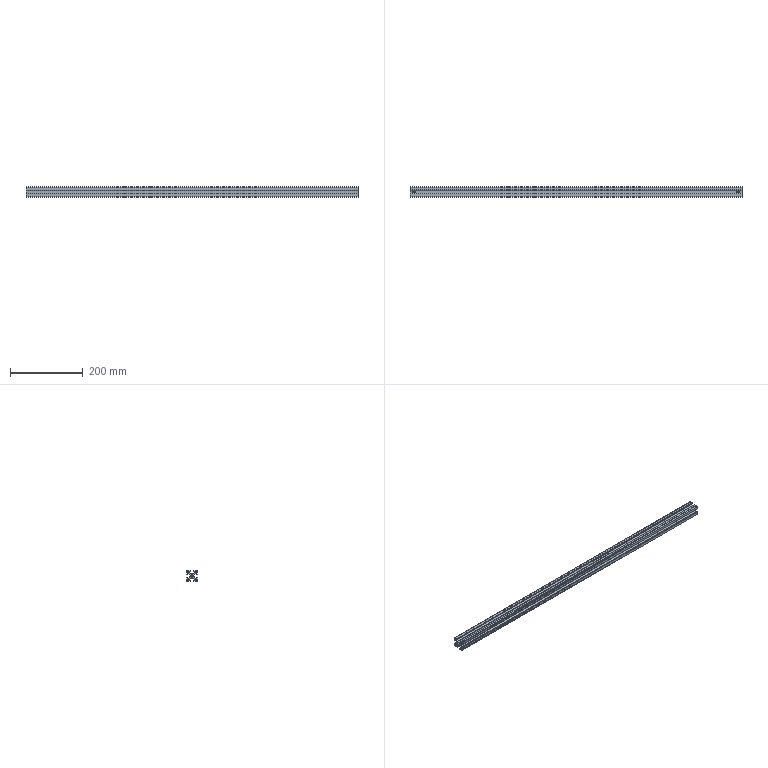Part | STEP file | MK-8-3030-L-99 profile 3030 standard 913mm | 1 solid | 163 faces | box 913 x 30 x 30 mm | volume 297727 mm3 | cylinder 85 | plane 78 | commonest cylinder face diameters 0.6 x55 2 x16 6.8 x6 5 x4 7 x4